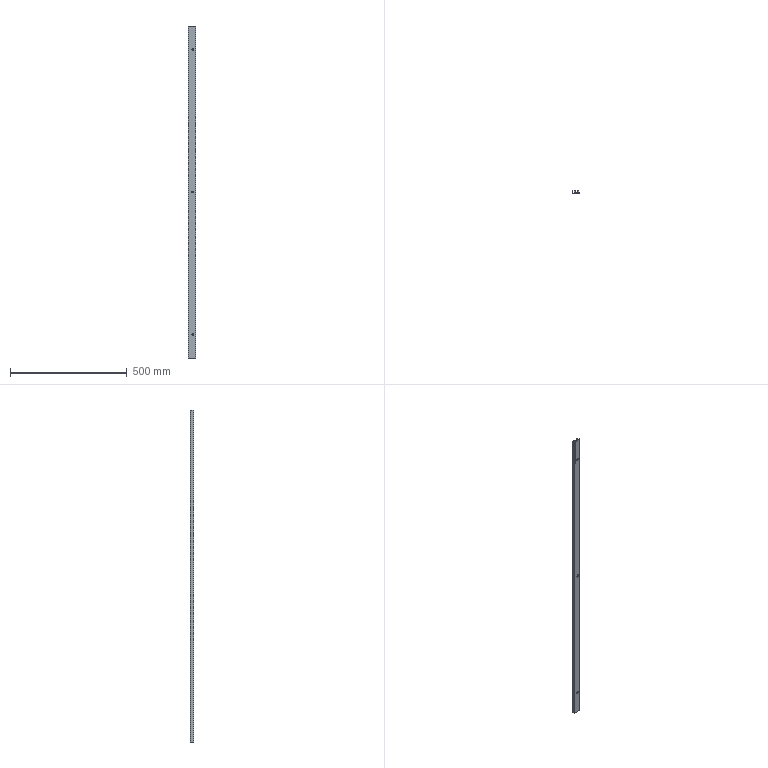Part | SolidWorks | features BaseBody 1, HoleWzd 1, ICE 1, MoveFace 1 | 1 solid | 31 faces | box 33.5 x 13.5 x 1420 mm | volume 265656 mm3 | plane 16 | cylinder 9 | cone 6 | commonest cylinder face diameters 2 x3 13.44 x3 4 x2 1.5 x1
STEP:
#1=CARTESIAN_POINT('',(20.,0.,1223.72));
#2=VERTEX_POINT('',#1);
#3=CARTESIAN_POINT('',(20.,0.,1216.28));
#4=VERTEX_POINT('',#3);
#5=CARTESIAN_POINT('',(20.,0.,1220.));
#6=DIRECTION('',(0.,-1.,0.));
#7=DIRECTION('',(0.,0.,-1.));
#8=AXIS2_PLACEMENT_3D('',#5,#6,#7);
#9=CIRCLE('',#8,3.72);
#10=EDGE_CURVE('',#2,#4,#9,.T.);
#11=ORIENTED_EDGE('',*,*,#10,.T.);
#12=CARTESIAN_POINT('',(20.,3.,1213.28));
#13=VERTEX_POINT('',#12);
#14=CARTESIAN_POINT('',(20.,3.,1213.28));
#15=DIRECTION('',(0.,0.7071,-0.7071));
#16=VECTOR('',#15,1000.);
#17=LINE('',#14,#16);
#18=EDGE_CURVE('',#4,#13,#17,.T.);
#19=ORIENTED_EDGE('',*,*,#18,.T.);
#20=CARTESIAN_POINT('',(20.,3.,1226.72));
#21=VERTEX_POINT('',#20);
#22=CARTESIAN_POINT('',(20.,3.,1220.));
#23=DIRECTION('',(0.,1.,0.));
#24=DIRECTION('',(0.,0.,1.));
#25=AXIS2_PLACEMENT_3D('',#22,#23,#24);
#26=CIRCLE('',#25,6.72);
#27=EDGE_CURVE('',#13,#21,#26,.T.);
#28=ORIENTED_EDGE('',*,*,#27,.T.);
#29=CARTESIAN_POINT('',(20.,3.,1226.72));
#30=DIRECTION('',(0.,0.7071,0.7071));
#31=VECTOR('',#30,1000.);
#32=LINE('',#29,#31);
#33=EDGE_CURVE('',#2,#21,#32,.T.);
#34=ORIENTED_EDGE('',*,*,#33,.F.);
#35=EDGE_LOOP('',(#11,#19,#28,#34));
#36=FACE_OUTER_BOUND('',#35,.T.);
#37=CARTESIAN_POINT('',(20.,3.,1220.));
#38=DIRECTION('',(0.,1.,0.));
#39=DIRECTION('',(0.,0.,1.));
#40=AXIS2_PLACEMENT_3D('',#37,#38,#39);
#41=CONICAL_SURFACE('',#40,6.72,0.7854);
#42=ADVANCED_FACE('',(#36),#41,.F.);
#43=CARTESIAN_POINT('',(20.,0.,3.72));
#44=VERTEX_POINT('',#43);
#45=CARTESIAN_POINT('',(20.,0.,-3.72));
#46=VERTEX_POINT('',#45);
#47=CARTESIAN_POINT('',(20.,0.,0.));
#48=DIRECTION('',(0.,-1.,0.));
#49=DIRECTION('',(0.,0.,-1.));
#50=AXIS2_PLACEMENT_3D('',#47,#48,#49);
#51=CIRCLE('',#50,3.72);
#52=EDGE_CURVE('',#44,#46,#51,.T.);
#53=ORIENTED_EDGE('',*,*,#52,.T.);
#54=CARTESIAN_POINT('',(20.,3.,-6.72));
#55=VERTEX_POINT('',#54);
#56=CARTESIAN_POINT('',(20.,3.,-6.72));
#57=DIRECTION('',(0.,0.7071,-0.7071));
#58=VECTOR('',#57,1000.);
#59=LINE('',#56,#58);
#60=EDGE_CURVE('',#46,#55,#59,.T.);
#61=ORIENTED_EDGE('',*,*,#60,.T.);
#62=CARTESIAN_POINT('',(20.,3.,6.72));
#63=VERTEX_POINT('',#62);
#64=CARTESIAN_POINT('',(20.,3.,0.));
#65=DIRECTION('',(0.,1.,0.));
#66=DIRECTION('',(0.,0.,1.));
#67=AXIS2_PLACEMENT_3D('',#64,#65,#66);
#68=CIRCLE('',#67,6.72);
#69=EDGE_CURVE('',#55,#63,#68,.T.);
#70=ORIENTED_EDGE('',*,*,#69,.T.);
#71=CARTESIAN_POINT('',(20.,3.,6.72));
#72=DIRECTION('',(0.,0.7071,0.7071));
#73=VECTOR('',#72,1000.);
#74=LINE('',#71,#73);
#75=EDGE_CURVE('',#44,#63,#74,.T.);
#76=ORIENTED_EDGE('',*,*,#75,.F.);
#77=EDGE_LOOP('',(#53,#61,#70,#76));
#78=FACE_OUTER_BOUND('',#77,.T.);
#79=CARTESIAN_POINT('',(20.,3.,0.));
#80=DIRECTION('',(0.,1.,0.));
#81=DIRECTION('',(0.,0.,1.));
#82=AXIS2_PLACEMENT_3D('',#79,#80,#81);
#83=CONICAL_SURFACE('',#82,6.72,0.7854);
#84=ADVANCED_FACE('',(#78),#83,.F.);
#85=CARTESIAN_POINT('',(20.,0.,613.72));
#86=VERTEX_POINT('',#85);
#87=CARTESIAN_POINT('',(20.,0.,606.28));
#88=VERTEX_POINT('',#87);
#89=CARTESIAN_POINT('',(20.,0.,610.));
#90=DIRECTION('',(0.,-1.,0.));
#91=DIRECTION('',(0.,0.,-1.));
#92=AXIS2_PLACEMENT_3D('',#89,#90,#91);
#93=CIRCLE('',#92,3.72);
#94=EDGE_CURVE('',#86,#88,#93,.T.);
#95=ORIENTED_EDGE('',*,*,#94,.T.);
#96=CARTESIAN_POINT('',(20.,3.,603.28));
#97=VERTEX_POINT('',#96);
#98=CARTESIAN_POINT('',(20.,3.,603.28));
#99=DIRECTION('',(0.,0.7071,-0.7071));
#100=VECTOR('',#99,1000.);
#101=LINE('',#98,#100);
#102=EDGE_CURVE('',#88,#97,#101,.T.);
#103=ORIENTED_EDGE('',*,*,#102,.T.);
#104=CARTESIAN_POINT('',(20.,3.,616.72));
#105=VERTEX_POINT('',#104);
#106=CARTESIAN_POINT('',(20.,3.,610.));
#107=DIRECTION('',(0.,1.,0.));
#108=DIRECTION('',(0.,0.,1.));
#109=AXIS2_PLACEMENT_3D('',#106,#107,#108);
#110=CIRCLE('',#109,6.72);
#111=EDGE_CURVE('',#97,#105,#110,.T.);
#112=ORIENTED_EDGE('',*,*,#111,.T.);
#113=CARTESIAN_POINT('',(20.,3.,616.72));
#114=DIRECTION('',(0.,0.7071,0.7071));
#115=VECTOR('',#114,1000.);
#116=LINE('',#113,#115);
#117=EDGE_CURVE('',#86,#105,#116,.T.);
#118=ORIENTED_EDGE('',*,*,#117,.F.);
#119=EDGE_LOOP('',(#95,#103,#112,#118));
#120=FACE_OUTER_BOUND('',#119,.T.);
#121=CARTESIAN_POINT('',(20.,3.,610.));
#122=DIRECTION('',(0.,1.,0.));
#123=DIRECTION('',(0.,0.,1.));
#124=AXIS2_PLACEMENT_3D('',#121,#122,#123);
#125=CONICAL_SURFACE('',#124,6.72,0.7854);
#126=ADVANCED_FACE('',(#120),#125,.F.);
#127=CARTESIAN_POINT('',(24.5,10.5,-4.991));
#128=VERTEX_POINT('',#127);
#129=CARTESIAN_POINT('',(24.5,10.5,-100.));
#130=VERTEX_POINT('',#129);
#131=CARTESIAN_POINT('',(24.5,10.5,-100.));
#132=DIRECTION('',(0.,0.,-1.));
#133=VECTOR('',#132,1000.);
#134=LINE('',#131,#133);
#135=EDGE_CURVE('',#128,#130,#134,.T.);
#136=ORIENTED_EDGE('',*,*,#135,.F.);
#137=CARTESIAN_POINT('',(24.5,10.5,4.991));
#138=VERTEX_POINT('',#137);
#139=CARTESIAN_POINT('',(24.5,10.5,-4.991));
#140=CARTESIAN_POINT('',(24.5,10.638,-4.991));
#141=CARTESIAN_POINT('',(24.515,10.777,-4.978));
#142=CARTESIAN_POINT('',(24.57,11.043,-4.927));
#143=CARTESIAN_POINT('',(24.611,11.171,-4.889));
#144=CARTESIAN_POINT('',(24.765,11.529,-4.74));
#145=CARTESIAN_POINT('',(24.907,11.728,-4.597));
#146=CARTESIAN_POINT('',(25.205,12.04,-4.256));
#147=CARTESIAN_POINT('',(25.365,12.156,-4.055));
#148=CARTESIAN_POINT('',(25.663,12.325,-3.627));
#149=CARTESIAN_POINT('',(25.806,12.38,-3.395));
#150=CARTESIAN_POINT('',(26.19,12.494,-2.672));
#151=CARTESIAN_POINT('',(26.387,12.501,-2.161));
#152=CARTESIAN_POINT('',(26.654,12.499,-1.091));
#153=CARTESIAN_POINT('',(26.72,12.488,-0.5481));
#154=CARTESIAN_POINT('',(26.72,12.488,0.2773));
#155=CARTESIAN_POINT('',(26.703,12.49,0.5529));
#156=CARTESIAN_POINT('',(26.636,12.496,1.095));
#157=CARTESIAN_POINT('',(26.586,12.499,1.362));
#158=CARTESIAN_POINT('',(26.388,12.501,2.155));
#159=CARTESIAN_POINT('',(26.188,12.493,2.677));
#160=CARTESIAN_POINT('',(25.805,12.38,3.396));
#161=CARTESIAN_POINT('',(25.662,12.324,3.629));
#162=CARTESIAN_POINT('',(25.438,12.197,3.95));
#163=CARTESIAN_POINT('',(25.362,12.147,4.053));
#164=CARTESIAN_POINT('',(25.208,12.03,4.249));
#165=CARTESIAN_POINT('',(25.13,11.961,4.342));
#166=CARTESIAN_POINT('',(24.98,11.805,4.513));
#167=CARTESIAN_POINT('',(24.908,11.717,4.591));
#168=CARTESIAN_POINT('',(24.774,11.518,4.73));
#169=CARTESIAN_POINT('',(24.714,11.408,4.79));
#170=CARTESIAN_POINT('',(24.612,11.172,4.888));
#171=CARTESIAN_POINT('',(24.57,11.043,4.927));
#172=CARTESIAN_POINT('',(24.515,10.778,4.978));
#173=CARTESIAN_POINT('',(24.5,10.64,4.991));
#174=CARTESIAN_POINT('',(24.5,10.5,4.991));
#175=B_SPLINE_CURVE_WITH_KNOTS('',3,(#139,#140,#141,#142,#143,#144,#145,#146,#147,#148,#149,#150,#151,#152,#153,#154,#155,#156,#157,#158,#159,#160,#161,#162,#163,#164,#165,#166,#167,#168,#169,#170,#171,#172,#173,#174),.UNSPECIFIED.,.F.,.F.,(4,2,2,2,2,2,2,2,2,2,2,2,2,2,2,2,2,4),(0.01321,0.01362,0.01403,0.01486,0.01569,0.01651,0.01816,0.01981,0.02064,0.02146,0.02311,0.02394,0.02435,0.02477,0.02518,0.02559,0.026,0.02642),.UNSPECIFIED.);
#176=EDGE_CURVE('',#128,#138,#175,.T.);
#177=ORIENTED_EDGE('',*,*,#176,.T.);
#178=CARTESIAN_POINT('',(24.5,10.5,605.009));
#179=VERTEX_POINT('',#178);
#180=CARTESIAN_POINT('',(24.5,10.5,-100.));
#181=DIRECTION('',(0.,0.,-1.));
#182=VECTOR('',#181,1000.);
#183=LINE('',#180,#182);
#184=EDGE_CURVE('',#179,#138,#183,.T.);
#185=ORIENTED_EDGE('',*,*,#184,.F.);
#186=CARTESIAN_POINT('',(24.5,10.5,614.991));
#187=VERTEX_POINT('',#186);
#188=CARTESIAN_POINT('',(24.5,10.5,605.009));
#189=CARTESIAN_POINT('',(24.5,10.638,605.009));
#190=CARTESIAN_POINT('',(24.515,10.777,605.022));
#191=CARTESIAN_POINT('',(24.57,11.043,605.073));
#192=CARTESIAN_POINT('',(24.611,11.171,605.111));
#193=CARTESIAN_POINT('',(24.765,11.529,605.26));
#194=CARTESIAN_POINT('',(24.907,11.728,605.403));
#195=CARTESIAN_POINT('',(25.205,12.04,605.744));
#196=CARTESIAN_POINT('',(25.365,12.156,605.945));
#197=CARTESIAN_POINT('',(25.663,12.325,606.373));
#198=CARTESIAN_POINT('',(25.806,12.38,606.605));
#199=CARTESIAN_POINT('',(26.19,12.494,607.328));
#200=CARTESIAN_POINT('',(26.387,12.501,607.839));
#201=CARTESIAN_POINT('',(26.654,12.499,608.909));
#202=CARTESIAN_POINT('',(26.72,12.488,609.452));
#203=CARTESIAN_POINT('',(26.72,12.488,610.277));
#204=CARTESIAN_POINT('',(26.703,12.49,610.553));
#205=CARTESIAN_POINT('',(26.636,12.496,611.095));
#206=CARTESIAN_POINT('',(26.586,12.499,611.362));
#207=CARTESIAN_POINT('',(26.388,12.501,612.155));
#208=CARTESIAN_POINT('',(26.188,12.493,612.677));
#209=CARTESIAN_POINT('',(25.805,12.38,613.396));
#210=CARTESIAN_POINT('',(25.662,12.324,613.629));
#211=CARTESIAN_POINT('',(25.438,12.197,613.95));
#212=CARTESIAN_POINT('',(25.362,12.147,614.053));
#213=CARTESIAN_POINT('',(25.208,12.03,614.249));
#214=CARTESIAN_POINT('',(25.13,11.961,614.342));
#215=CARTESIAN_POINT('',(24.98,11.805,614.513));
#216=CARTESIAN_POINT('',(24.908,11.717,614.591));
#217=CARTESIAN_POINT('',(24.774,11.518,614.73));
#218=CARTESIAN_POINT('',(24.714,11.408,614.79));
#219=CARTESIAN_POINT('',(24.612,11.172,614.888));
#220=CARTESIAN_POINT('',(24.57,11.043,614.927));
#221=CARTESIAN_POINT('',(24.515,10.778,614.978));
#222=CARTESIAN_POINT('',(24.5,10.64,614.991));
#223=CARTESIAN_POINT('',(24.5,10.5,614.991));
#224=B_SPLINE_CURVE_WITH_KNOTS('',3,(#188,#189,#190,#191,#192,#193,#194,#195,#196,#197,#198,#199,#200,#201,#202,#203,#204,#205,#206,#207,#208,#209,#210,#211,#212,#213,#214,#215,#216,#217,#218,#219,#220,#221,#222,#223),.UNSPECIFIED.,.F.,.F.,(4,2,2,2,2,2,2,2,2,2,2,2,2,2,2,2,2,4),(0.01321,0.01362,0.01403,0.01486,0.01569,0.01651,0.01816,0.01981,0.02064,0.02146,0.02311,0.02394,0.02435,0.02477,0.02518,0.02559,0.026,0.02642),.UNSPECIFIED.);
#225=EDGE_CURVE('',#179,#187,#224,.T.);
#226=ORIENTED_EDGE('',*,*,#225,.T.);
#227=CARTESIAN_POINT('',(24.5,10.5,1215.009));
#228=VERTEX_POINT('',#227);
#229=CARTESIAN_POINT('',(24.5,10.5,-100.));
#230=DIRECTION('',(0.,0.,-1.));
#231=VECTOR('',#230,1000.);
#232=LINE('',#229,#231);
#233=EDGE_CURVE('',#228,#187,#232,.T.);
#234=ORIENTED_EDGE('',*,*,#233,.F.);
#235=CARTESIAN_POINT('',(24.5,10.5,1224.991));
#236=VERTEX_POINT('',#235);
#237=CARTESIAN_POINT('',(24.5,10.5,1215.009));
#238=CARTESIAN_POINT('',(24.5,10.64,1215.009));
#239=CARTESIAN_POINT('',(24.514,10.776,1215.022));
#240=CARTESIAN_POINT('',(24.57,11.042,1215.073));
#241=CARTESIAN_POINT('',(24.611,11.171,1215.111));
#242=CARTESIAN_POINT('',(24.713,11.408,1215.209));
#243=CARTESIAN_POINT('',(24.775,11.519,1215.27));
#244=CARTESIAN_POINT('',(24.908,11.717,1215.409));
#245=CARTESIAN_POINT('',(24.981,11.806,1215.488));
#246=CARTESIAN_POINT('',(25.207,12.042,1215.746));
#247=CARTESIAN_POINT('',(25.363,12.155,1215.942));
#248=CARTESIAN_POINT('',(25.665,12.326,1216.376));
#249=CARTESIAN_POINT('',(25.806,12.38,1216.605));
#250=CARTESIAN_POINT('',(26.061,12.456,1217.084));
#251=CARTESIAN_POINT('',(26.176,12.476,1217.337));
#252=CARTESIAN_POINT('',(26.372,12.498,1217.849));
#253=CARTESIAN_POINT('',(26.454,12.501,1218.109));
#254=CARTESIAN_POINT('',(26.586,12.499,1218.638));
#255=CARTESIAN_POINT('',(26.636,12.496,1218.907));
#256=CARTESIAN_POINT('',(26.703,12.49,1219.453));
#257=CARTESIAN_POINT('',(26.72,12.488,1219.729));
#258=CARTESIAN_POINT('',(26.72,12.488,1220.275));
#259=CARTESIAN_POINT('',(26.703,12.49,1220.547));
#260=CARTESIAN_POINT('',(26.637,12.496,1221.089));
#261=CARTESIAN_POINT('',(26.587,12.499,1221.36));
#262=CARTESIAN_POINT('',(26.387,12.501,1222.161));
#263=CARTESIAN_POINT('',(26.191,12.494,1222.671));
#264=CARTESIAN_POINT('',(25.805,12.38,1223.396));
#265=CARTESIAN_POINT('',(25.663,12.325,1223.627));
#266=CARTESIAN_POINT('',(25.364,12.155,1224.057));
#267=CARTESIAN_POINT('',(25.205,12.039,1224.256));
#268=CARTESIAN_POINT('',(24.981,11.805,1224.512));
#269=CARTESIAN_POINT('',(24.907,11.716,1224.592));
#270=CARTESIAN_POINT('',(24.774,11.518,1224.73));
#271=CARTESIAN_POINT('',(24.714,11.409,1224.79));
#272=CARTESIAN_POINT('',(24.611,11.17,1224.889));
#273=CARTESIAN_POINT('',(24.571,11.044,1224.926));
#274=CARTESIAN_POINT('',(24.515,10.78,1224.977));
#275=CARTESIAN_POINT('',(24.5,10.64,1224.991));
#276=CARTESIAN_POINT('',(24.5,10.5,1224.991));
#277=B_SPLINE_CURVE_WITH_KNOTS('',3,(#237,#238,#239,#240,#241,#242,#243,#244,#245,#246,#247,#248,#249,#250,#251,#252,#253,#254,#255,#256,#257,#258,#259,#260,#261,#262,#263,#264,#265,#266,#267,#268,#269,#270,#271,#272,#273,#274,#275,#276),.UNSPECIFIED.,.F.,.F.,(4,2,2,2,2,2,2,2,2,2,2,2,2,2,2,2,2,2,2,4),(0.,0.0004127,0.0008255,0.001238,0.001651,0.002476,0.003302,0.004127,0.004953,0.005778,0.006604,0.007429,0.008255,0.009906,0.01073,0.01156,0.01197,0.01238,0.01279,0.01321),.UNSPECIFIED.);
#278=EDGE_CURVE('',#228,#236,#277,.T.);
#279=ORIENTED_EDGE('',*,*,#278,.T.);
#280=CARTESIAN_POINT('',(24.5,10.5,1320.));
#281=VERTEX_POINT('',#280);
#282=CARTESIAN_POINT('',(24.5,10.5,-100.));
#283=DIRECTION('',(0.,0.,-1.));
#284=VECTOR('',#283,1000.);
#285=LINE('',#282,#284);
#286=EDGE_CURVE('',#281,#236,#285,.T.);
#287=ORIENTED_EDGE('',*,*,#286,.F.);
#288=CARTESIAN_POINT('',(28.5,10.5,1320.));
#289=VERTEX_POINT('',#288);
#290=CARTESIAN_POINT('',(26.5,10.5,1320.));
#291=DIRECTION('',(0.,0.,1.));
#292=DIRECTION('',(1.,0.,0.));
#293=AXIS2_PLACEMENT_3D('',#290,#291,#292);
#294=CIRCLE('',#293,2.);
#295=EDGE_CURVE('',#289,#281,#294,.T.);
#296=ORIENTED_EDGE('',*,*,#295,.F.);
#297=CARTESIAN_POINT('',(28.5,10.5,-100.));
#298=VERTEX_POINT('',#297);
#299=CARTESIAN_POINT('',(28.5,10.5,-100.));
#300=DIRECTION('',(0.,0.,-1.));
#301=VECTOR('',#300,1000.);
#302=LINE('',#299,#301);
#303=EDGE_CURVE('',#289,#298,#302,.T.);
#304=ORIENTED_EDGE('',*,*,#303,.T.);
#305=CARTESIAN_POINT('',(26.5,10.5,-100.));
#306=DIRECTION('',(0.,0.,1.));
#307=DIRECTION('',(-1.,0.,0.));
#308=AXIS2_PLACEMENT_3D('',#305,#306,#307);
#309=CIRCLE('',#308,2.);
#310=EDGE_CURVE('',#298,#130,#309,.T.);
#311=ORIENTED_EDGE('',*,*,#310,.T.);
#312=EDGE_LOOP('',(#136,#177,#185,#226,#234,#279,#287,#296,#304,#311));
#313=FACE_OUTER_BOUND('',#312,.T.);
#314=CARTESIAN_POINT('',(26.5,10.5,-100.));
#315=DIRECTION('',(0.,0.,-1.));
#316=DIRECTION('',(-1.,0.,0.));
#317=AXIS2_PLACEMENT_3D('',#314,#315,#316);
#318=CYLINDRICAL_SURFACE('',#317,2.);
#319=ADVANCED_FACE('',(#313),#318,.T.);
#320=CARTESIAN_POINT('',(24.5,3.,-4.991));
#321=VERTEX_POINT('',#320);
#322=CARTESIAN_POINT('',(24.5,3.,-100.));
#323=VERTEX_POINT('',#322);
#324=CARTESIAN_POINT('',(24.5,3.,-100.));
#325=DIRECTION('',(0.,0.,-1.));
#326=VECTOR('',#325,1000.);
#327=LINE('',#324,#326);
#328=EDGE_CURVE('',#321,#323,#327,.T.);
#329=ORIENTED_EDGE('',*,*,#328,.F.);
#330=CARTESIAN_POINT('',(24.5,13.5,-4.991));
#331=DIRECTION('',(0.,1.,0.));
#332=VECTOR('',#331,1000.);
#333=LINE('',#330,#332);
#334=EDGE_CURVE('',#321,#128,#333,.T.);
#335=ORIENTED_EDGE('',*,*,#334,.T.);
#336=ORIENTED_EDGE('',*,*,#135,.T.);
#337=CARTESIAN_POINT('',(24.5,1.,-100.));
#338=DIRECTION('',(0.,-1.,0.));
#339=VECTOR('',#338,1000.);
#340=LINE('',#337,#339);
#341=EDGE_CURVE('',#130,#323,#340,.T.);
#342=ORIENTED_EDGE('',*,*,#341,.T.);
#343=EDGE_LOOP('',(#329,#335,#336,#342));
#344=FACE_OUTER_BOUND('',#343,.T.);
#345=CARTESIAN_POINT('',(24.5,10.5,-100.));
#346=DIRECTION('',(-1.,0.,0.));
#347=DIRECTION('',(0.,0.,1.));
#348=AXIS2_PLACEMENT_3D('',#345,#346,#347);
#349=PLANE('',#348);
#350=ADVANCED_FACE('',(#344),#349,.T.);
#351=ORIENTED_EDGE('',*,*,#184,.T.);
#352=CARTESIAN_POINT('',(24.5,3.,4.991));
#353=VERTEX_POINT('',#352);
#354=CARTESIAN_POINT('',(24.5,13.5,4.991));
#355=DIRECTION('',(0.,-1.,0.));
#356=VECTOR('',#355,1000.);
#357=LINE('',#354,#356);
#358=EDGE_CURVE('',#138,#353,#357,.T.);
#359=ORIENTED_EDGE('',*,*,#358,.T.);
#360=CARTESIAN_POINT('',(24.5,3.,605.009));
#361=VERTEX_POINT('',#360);
#362=CARTESIAN_POINT('',(24.5,3.,-100.));
#363=DIRECTION('',(0.,0.,-1.));
#364=VECTOR('',#363,1000.);
#365=LINE('',#362,#364);
#366=EDGE_CURVE('',#361,#353,#365,.T.);
#367=ORIENTED_EDGE('',*,*,#366,.F.);
#368=CARTESIAN_POINT('',(24.5,13.5,605.009));
#369=DIRECTION('',(0.,1.,0.));
#370=VECTOR('',#369,1000.);
#371=LINE('',#368,#370);
#372=EDGE_CURVE('',#361,#179,#371,.T.);
#373=ORIENTED_EDGE('',*,*,#372,.T.);
#374=EDGE_LOOP('',(#351,#359,#367,#373));
#375=FACE_OUTER_BOUND('',#374,.T.);
#376=CARTESIAN_POINT('',(24.5,10.5,-100.));
#377=DIRECTION('',(-1.,0.,0.));
#378=DIRECTION('',(0.,0.,1.));
#379=AXIS2_PLACEMENT_3D('',#376,#377,#378);
#380=PLANE('',#379);
#381=ADVANCED_FACE('',(#375),#380,.T.);
#382=ORIENTED_EDGE('',*,*,#233,.T.);
#383=CARTESIAN_POINT('',(24.5,3.,614.991));
#384=VERTEX_POINT('',#383);
#385=CARTESIAN_POINT('',(24.5,13.5,614.991));
#386=DIRECTION('',(0.,-1.,0.));
#387=VECTOR('',#386,1000.);
#388=LINE('',#385,#387);
#389=EDGE_CURVE('',#187,#384,#388,.T.);
#390=ORIENTED_EDGE('',*,*,#389,.T.);
#391=CARTESIAN_POINT('',(24.5,3.,1215.009));
#392=VERTEX_POINT('',#391);
#393=CARTESIAN_POINT('',(24.5,3.,-100.));
#394=DIRECTION('',(0.,0.,-1.));
#395=VECTOR('',#394,1000.);
#396=LINE('',#393,#395);
#397=EDGE_CURVE('',#392,#384,#396,.T.);
#398=ORIENTED_EDGE('',*,*,#397,.F.);
#399=CARTESIAN_POINT('',(24.5,13.5,1215.009));
#400=DIRECTION('',(0.,1.,0.));
#401=VECTOR('',#400,1000.);
#402=LINE('',#399,#401);
#403=EDGE_CURVE('',#392,#228,#402,.T.);
#404=ORIENTED_EDGE('',*,*,#403,.T.);
#405=EDGE_LOOP('',(#382,#390,#398,#404));
#406=FACE_OUTER_BOUND('',#405,.T.);
#407=CARTESIAN_POINT('',(24.5,10.5,-100.));
#408=DIRECTION('',(-1.,0.,0.));
#409=DIRECTION('',(0.,0.,1.));
#410=AXIS2_PLACEMENT_3D('',#407,#408,#409);
#411=PLANE('',#410);
#412=ADVANCED_FACE('',(#406),#411,.T.);
#413=ORIENTED_EDGE('',*,*,#286,.T.);
#414=CARTESIAN_POINT('',(24.5,3.,1224.991));
#415=VERTEX_POINT('',#414);
#416=CARTESIAN_POINT('',(24.5,13.5,1224.991));
#417=DIRECTION('',(0.,-1.,0.));
#418=VECTOR('',#417,1000.);
#419=LINE('',#416,#418);
#420=EDGE_CURVE('',#236,#415,#419,.T.);
#421=ORIENTED_EDGE('',*,*,#420,.T.);
#422=CARTESIAN_POINT('',(24.5,3.,1320.));
#423=VERTEX_POINT('',#422);
#424=CARTESIAN_POINT('',(24.5,3.,-100.));
#425=DIRECTION('',(0.,0.,-1.));
#426=VECTOR('',#425,1000.);
#427=LINE('',#424,#426);
#428=EDGE_CURVE('',#423,#415,#427,.T.);
#429=ORIENTED_EDGE('',*,*,#428,.F.);
#430=CARTESIAN_POINT('',(24.5,1.,1320.));
#431=DIRECTION('',(0.,-1.,0.));
#432=VECTOR('',#431,1000.);
#433=LINE('',#430,#432);
#434=EDGE_CURVE('',#281,#423,#433,.T.);
#435=ORIENTED_EDGE('',*,*,#434,.F.);
#436=EDGE_LOOP('',(#413,#421,#429,#435));
#437=FACE_OUTER_BOUND('',#436,.T.);
#438=CARTESIAN_POINT('',(24.5,10.5,-100.));
#439=DIRECTION('',(-1.,0.,0.));
#440=DIRECTION('',(0.,0.,1.));
#441=AXIS2_PLACEMENT_3D('',#438,#439,#440);
#442=PLANE('',#441);
#443=ADVANCED_FACE('',(#437),#442,.T.);
#444=ORIENTED_EDGE('',*,*,#10,.F.);
#445=CARTESIAN_POINT('',(20.,0.,1220.));
#446=DIRECTION('',(0.,-1.,0.));
#447=DIRECTION('',(0.,0.,-1.));
#448=AXIS2_PLACEMENT_3D('',#445,#446,#447);
#449=CIRCLE('',#448,3.72);
#450=EDGE_CURVE('',#4,#2,#449,.T.);
#451=ORIENTED_EDGE('',*,*,#450,.F.);
#452=EDGE_LOOP('',(#444,#451));
#453=FACE_BOUND('',#452,.T.);
#454=ORIENTED_EDGE('',*,*,#94,.F.);
#455=CARTESIAN_POINT('',(20.,0.,610.));
#456=DIRECTION('',(0.,-1.,0.));
#457=DIRECTION('',(0.,0.,-1.));
#458=AXIS2_PLACEMENT_3D('',#455,#456,#457);
#459=CIRCLE('',#458,3.72);
#460=EDGE_CURVE('',#88,#86,#459,.T.);
#461=ORIENTED_EDGE('',*,*,#460,.F.);
#462=EDGE_LOOP('',(#454,#461));
#463=FACE_BOUND('',#462,.T.);
#464=CARTESIAN_POINT('',(1.,0.,-100.));
#465=VERTEX_POINT('',#464);
#466=CARTESIAN_POINT('',(32.5,0.,-100.));
#467=VERTEX_POINT('',#466);
#468=CARTESIAN_POINT('',(1.,0.,-100.));
#469=DIRECTION('',(1.,0.,0.));
#470=VECTOR('',#469,1000.);
#471=LINE('',#468,#470);
#472=EDGE_CURVE('',#465,#467,#471,.T.);
#473=ORIENTED_EDGE('',*,*,#472,.T.);
#474=CARTESIAN_POINT('',(32.5,0.,1320.));
#475=VERTEX_POINT('',#474);
#476=CARTESIAN_POINT('',(32.5,0.,-100.));
#477=DIRECTION('',(0.,0.,1.));
#478=VECTOR('',#477,1000.);
#479=LINE('',#476,#478);
#480=EDGE_CURVE('',#467,#475,#479,.T.);
#481=ORIENTED_EDGE('',*,*,#480,.T.);
#482=CARTESIAN_POINT('',(1.,0.,1320.));
#483=VERTEX_POINT('',#482);
#484=CARTESIAN_POINT('',(1.,0.,1320.));
#485=DIRECTION('',(-1.,0.,0.));
#486=VECTOR('',#485,1000.);
#487=LINE('',#484,#486);
#488=EDGE_CURVE('',#475,#483,#487,.T.);
#489=ORIENTED_EDGE('',*,*,#488,.T.);
#490=CARTESIAN_POINT('',(1.,0.,-100.));
#491=DIRECTION('',(0.,0.,-1.));
#492=VECTOR('',#491,1000.);
#493=LINE('',#490,#492);
#494=EDGE_CURVE('',#483,#465,#493,.T.);
#495=ORIENTED_EDGE('',*,*,#494,.T.);
#496=EDGE_LOOP('',(#473,#481,#489,#495));
#497=FACE_OUTER_BOUND('',#496,.T.);
#498=ORIENTED_EDGE('',*,*,#52,.F.);
#499=CARTESIAN_POINT('',(20.,0.,0.));
#500=DIRECTION('',(0.,-1.,0.));
#501=DIRECTION('',(0.,0.,-1.));
#502=AXIS2_PLACEMENT_3D('',#499,#500,#501);
#503=CIRCLE('',#502,3.72);
#504=EDGE_CURVE('',#46,#44,#503,.T.);
#505=ORIENTED_EDGE('',*,*,#504,.F.);
#506=EDGE_LOOP('',(#498,#505));
#507=FACE_BOUND('',#506,.T.);
#508=CARTESIAN_POINT('',(1.,0.,-100.));
#509=DIRECTION('',(0.,-1.,0.));
#510=DIRECTION('',(0.,0.,-1.));
#511=AXIS2_PLACEMENT_3D('',#508,#509,#510);
#512=PLANE('',#511);
#513=ADVANCED_FACE('',(#453,#463,#497,#507),#512,.T.);
#514=CARTESIAN_POINT('',(33.5,1.,-100.));
#515=VERTEX_POINT('',#514);
#516=CARTESIAN_POINT('',(32.5,1.,-100.));
#517=DIRECTION('',(0.,0.,1.));
#518=DIRECTION('',(-1.,0.,0.));
#519=AXIS2_PLACEMENT_3D('',#516,#517,#518);
#520=CIRCLE('',#519,1.);
#521=EDGE_CURVE('',#467,#515,#520,.T.);
#522=ORIENTED_EDGE('',*,*,#521,.T.);
#523=CARTESIAN_POINT('',(33.5,1.,1320.));
#524=VERTEX_POINT('',#523);
#525=CARTESIAN_POINT('',(33.5,1.,-100.));
#526=DIRECTION('',(0.,0.,1.));
#527=VECTOR('',#526,1000.);
#528=LINE('',#525,#527);
#529=EDGE_CURVE('',#515,#524,#528,.T.);
#530=ORIENTED_EDGE('',*,*,#529,.T.);
#531=CARTESIAN_POINT('',(32.5,1.,1320.));
#532=DIRECTION('',(0.,0.,-1.));
#533=DIRECTION('',(1.,0.,0.));
#534=AXIS2_PLACEMENT_3D('',#531,#532,#533);
#535=CIRCLE('',#534,1.);
#536=EDGE_CURVE('',#524,#475,#535,.T.);
#537=ORIENTED_EDGE('',*,*,#536,.T.);
#538=ORIENTED_EDGE('',*,*,#480,.F.);
#539=EDGE_LOOP('',(#522,#530,#537,#538));
#540=FACE_OUTER_BOUND('',#539,.T.);
#541=CARTESIAN_POINT('',(32.5,1.,-100.));
#542=DIRECTION('',(0.,0.,-1.));
#543=DIRECTION('',(-1.,0.,0.));
#544=AXIS2_PLACEMENT_3D('',#541,#542,#543);
#545=CYLINDRICAL_SURFACE('',#544,1.);
#546=ADVANCED_FACE('',(#540),#545,.T.);
#547=CARTESIAN_POINT('',(1.5,12.75,-100.));
#548=VERTEX_POINT('',#547);
#549=CARTESIAN_POINT('',(0.,12.75,-100.));
#550=VERTEX_POINT('',#549);
#551=CARTESIAN_POINT('',(0.75,12.75,-100.));
#552=DIRECTION('',(0.,0.,1.));
#553=DIRECTION('',(-1.,0.,0.));
#554=AXIS2_PLACEMENT_3D('',#551,#552,#553);
#555=CIRCLE('',#554,0.75);
#556=EDGE_CURVE('',#548,#550,#555,.T.);
#557=ORIENTED_EDGE('',*,*,#556,.F.);
#558=CARTESIAN_POINT('',(1.5,3.,-100.));
#559=VERTEX_POINT('',#558);
#560=CARTESIAN_POINT('',(1.5,1.,-100.));
#561=DIRECTION('',(0.,1.,0.));
#562=VECTOR('',#561,1000.);
#563=LINE('',#560,#562);
#564=EDGE_CURVE('',#559,#548,#563,.T.);
#565=ORIENTED_EDGE('',*,*,#564,.F.);
#566=CARTESIAN_POINT('',(8.5,3.,-100.));
#567=VERTEX_POINT('',#566);
#568=CARTESIAN_POINT('',(1.,3.,-100.));
#569=DIRECTION('',(-1.,0.,0.));
#570=VECTOR('',#569,1000.);
#571=LINE('',#568,#570);
#572=EDGE_CURVE('',#567,#559,#571,.T.);
#573=ORIENTED_EDGE('',*,*,#572,.F.);
#574=CARTESIAN_POINT('',(8.5,10.5,-100.));
#575=VERTEX_POINT('',#574);
#576=CARTESIAN_POINT('',(8.5,1.,-100.));
#577=DIRECTION('',(0.,-1.,0.));
#578=VECTOR('',#577,1000.);
#579=LINE('',#576,#578);
#580=EDGE_CURVE('',#575,#567,#579,.T.);
#581=ORIENTED_EDGE('',*,*,#580,.F.);
#582=CARTESIAN_POINT('',(12.5,10.5,-100.));
#583=VERTEX_POINT('',#582);
#584=CARTESIAN_POINT('',(10.5,10.5,-100.));
#585=DIRECTION('',(0.,0.,1.));
#586=DIRECTION('',(-1.,0.,0.));
#587=AXIS2_PLACEMENT_3D('',#584,#585,#586);
#588=CIRCLE('',#587,2.);
#589=EDGE_CURVE('',#583,#575,#588,.T.);
#590=ORIENTED_EDGE('',*,*,#589,.F.);
#591=CARTESIAN_POINT('',(12.5,3.,-100.));
#592=VERTEX_POINT('',#591);
#593=CARTESIAN_POINT('',(12.5,1.,-100.));
#594=DIRECTION('',(0.,1.,0.));
#595=VECTOR('',#594,1000.);
#596=LINE('',#593,#595);
#597=EDGE_CURVE('',#592,#583,#596,.T.);
#598=ORIENTED_EDGE('',*,*,#597,.F.);
#599=CARTESIAN_POINT('',(1.,3.,-100.));
#600=DIRECTION('',(-1.,0.,0.));
#601=VECTOR('',#600,1000.);
#602=LINE('',#599,#601);
#603=EDGE_CURVE('',#323,#592,#602,.T.);
#604=ORIENTED_EDGE('',*,*,#603,.F.);
#605=ORIENTED_EDGE('',*,*,#341,.F.);
#606=ORIENTED_EDGE('',*,*,#310,.F.);
#607=CARTESIAN_POINT('',(28.5,3.,-100.));
#608=VERTEX_POINT('',#607);
#609=CARTESIAN_POINT('',(28.5,1.,-100.));
#610=DIRECTION('',(0.,1.,0.));
#611=VECTOR('',#610,1000.);
#612=LINE('',#609,#611);
#613=EDGE_CURVE('',#608,#298,#612,.T.);
#614=ORIENTED_EDGE('',*,*,#613,.F.);
#615=CARTESIAN_POINT('',(32.5,3.,-100.));
#616=VERTEX_POINT('',#615);
#617=CARTESIAN_POINT('',(1.,3.,-100.));
#618=DIRECTION('',(-1.,0.,0.));
#619=VECTOR('',#618,1000.);
#620=LINE('',#617,#619);
#621=EDGE_CURVE('',#616,#608,#620,.T.);
#622=ORIENTED_EDGE('',*,*,#621,.F.);
#623=CARTESIAN_POINT('',(33.5,2.,-100.));
#624=VERTEX_POINT('',#623);
#625=CARTESIAN_POINT('',(32.5,2.,-100.));
#626=DIRECTION('',(0.,0.,1.));
#627=DIRECTION('',(-1.,0.,0.));
#628=AXIS2_PLACEMENT_3D('',#625,#626,#627);
#629=CIRCLE('',#628,1.);
#630=EDGE_CURVE('',#624,#616,#629,.T.);
#631=ORIENTED_EDGE('',*,*,#630,.F.);
#632=CARTESIAN_POINT('',(33.5,1.,-100.));
#633=DIRECTION('',(0.,1.,0.));
#634=VECTOR('',#633,1000.);
#635=LINE('',#632,#634);
#636=EDGE_CURVE('',#515,#624,#635,.T.);
#637=ORIENTED_EDGE('',*,*,#636,.F.);
#638=ORIENTED_EDGE('',*,*,#521,.F.);
#639=ORIENTED_EDGE('',*,*,#472,.F.);
#640=CARTESIAN_POINT('',(0.,1.,-100.));
#641=VERTEX_POINT('',#640);
#642=CARTESIAN_POINT('',(1.,1.,-100.));
#643=DIRECTION('',(0.,0.,1.));
#644=DIRECTION('',(-1.,0.,0.));
#645=AXIS2_PLACEMENT_3D('',#642,#643,#644);
#646=CIRCLE('',#645,1.);
#647=EDGE_CURVE('',#641,#465,#646,.T.);
#648=ORIENTED_EDGE('',*,*,#647,.F.);
#649=CARTESIAN_POINT('',(0.,1.,-100.));
#650=DIRECTION('',(0.,-1.,0.));
#651=VECTOR('',#650,1000.);
#652=LINE('',#649,#651);
#653=EDGE_CURVE('',#550,#641,#652,.T.);
#654=ORIENTED_EDGE('',*,*,#653,.F.);
#655=EDGE_LOOP('',(#557,#565,#573,#581,#590,#598,#604,#605,#606,#614,#622,#631,#637,#638,#639,#648,#654));
#656=FACE_OUTER_BOUND('',#655,.T.);
#657=CARTESIAN_POINT('',(1.,1.,-100.));
#658=DIRECTION('',(0.,0.,1.));
#659=DIRECTION('',(1.,0.,0.));
#660=AXIS2_PLACEMENT_3D('',#657,#658,#659);
#661=PLANE('',#660);
#662=ADVANCED_FACE('',(#656),#661,.F.);
#663=ORIENTED_EDGE('',*,*,#647,.T.);
#664=ORIENTED_EDGE('',*,*,#494,.F.);
#665=CARTESIAN_POINT('',(0.,1.,1320.));
#666=VERTEX_POINT('',#665);
#667=CARTESIAN_POINT('',(1.,1.,1320.));
#668=DIRECTION('',(0.,0.,-1.));
#669=DIRECTION('',(1.,0.,0.));
#670=AXIS2_PLACEMENT_3D('',#667,#668,#669);
#671=CIRCLE('',#670,1.);
#672=EDGE_CURVE('',#483,#666,#671,.T.);
#673=ORIENTED_EDGE('',*,*,#672,.T.);
#674=CARTESIAN_POINT('',(0.,1.,-100.));
#675=DIRECTION('',(0.,0.,-1.));
#676=VECTOR('',#675,1000.);
#677=LINE('',#674,#676);
#678=EDGE_CURVE('',#666,#641,#677,.T.);
#679=ORIENTED_EDGE('',*,*,#678,.T.);
#680=EDGE_LOOP('',(#663,#664,#673,#679));
#681=FACE_OUTER_BOUND('',#680,.T.);
#682=CARTESIAN_POINT('',(1.,1.,-100.));
#683=DIRECTION('',(0.,0.,-1.));
#684=DIRECTION('',(-1.,0.,0.));
#685=AXIS2_PLACEMENT_3D('',#682,#683,#684);
#686=CYLINDRICAL_SURFACE('',#685,1.);
#687=ADVANCED_FACE('',(#681),#686,.T.);
#688=CARTESIAN_POINT('',(1.5,3.,1320.));
#689=VERTEX_POINT('',#688);
#690=CARTESIAN_POINT('',(1.5,12.75,1320.));
#691=VERTEX_POINT('',#690);
#692=CARTESIAN_POINT('',(1.5,1.,1320.));
#693=DIRECTION('',(0.,1.,0.));
#694=VECTOR('',#693,1000.);
#695=LINE('',#692,#694);
#696=EDGE_CURVE('',#689,#691,#695,.T.);
#697=ORIENTED_EDGE('',*,*,#696,.T.);
#698=CARTESIAN_POINT('',(0.,12.75,1320.));
#699=VERTEX_POINT('',#698);
#700=CARTESIAN_POINT('',(0.75,12.75,1320.));
#701=DIRECTION('',(0.,0.,1.));
#702=DIRECTION('',(1.,0.,0.));
#703=AXIS2_PLACEMENT_3D('',#700,#701,#702);
#704=CIRCLE('',#703,0.75);
#705=EDGE_CURVE('',#691,#699,#704,.T.);
#706=ORIENTED_EDGE('',*,*,#705,.T.);
#707=CARTESIAN_POINT('',(0.,1.,1320.));
#708=DIRECTION('',(0.,-1.,0.));
#709=VECTOR('',#708,1000.);
#710=LINE('',#707,#709);
#711=EDGE_CURVE('',#699,#666,#710,.T.);
#712=ORIENTED_EDGE('',*,*,#711,.T.);
#713=ORIENTED_EDGE('',*,*,#672,.F.);
#714=ORIENTED_EDGE('',*,*,#488,.F.);
#715=ORIENTED_EDGE('',*,*,#536,.F.);
#716=CARTESIAN_POINT('',(33.5,2.,1320.));
#717=VERTEX_POINT('',#716);
#718=CARTESIAN_POINT('',(33.5,1.,1320.));
#719=DIRECTION('',(0.,1.,0.));
#720=VECTOR('',#719,1000.);
#721=LINE('',#718,#720);
#722=EDGE_CURVE('',#524,#717,#721,.T.);
#723=ORIENTED_EDGE('',*,*,#722,.T.);
#724=CARTESIAN_POINT('',(32.5,3.,1320.));
#725=VERTEX_POINT('',#724);
#726=CARTESIAN_POINT('',(32.5,2.,1320.));
#727=DIRECTION('',(0.,0.,-1.));
#728=DIRECTION('',(1.,0.,0.));
#729=AXIS2_PLACEMENT_3D('',#726,#727,#728);
#730=CIRCLE('',#729,1.);
#731=EDGE_CURVE('',#725,#717,#730,.T.);
#732=ORIENTED_EDGE('',*,*,#731,.F.);
#733=CARTESIAN_POINT('',(28.5,3.,1320.));
#734=VERTEX_POINT('',#733);
#735=CARTESIAN_POINT('',(1.,3.,1320.));
#736=DIRECTION('',(-1.,0.,0.));
#737=VECTOR('',#736,1000.);
#738=LINE('',#735,#737);
#739=EDGE_CURVE('',#725,#734,#738,.T.);
#740=ORIENTED_EDGE('',*,*,#739,.T.);
#741=CARTESIAN_POINT('',(28.5,1.,1320.));
#742=DIRECTION('',(0.,1.,0.));
#743=VECTOR('',#742,1000.);
#744=LINE('',#741,#743);
#745=EDGE_CURVE('',#734,#289,#744,.T.);
#746=ORIENTED_EDGE('',*,*,#745,.T.);
#747=ORIENTED_EDGE('',*,*,#295,.T.);
#748=ORIENTED_EDGE('',*,*,#434,.T.);
#749=CARTESIAN_POINT('',(12.5,3.,1320.));
#750=VERTEX_POINT('',#749);
#751=CARTESIAN_POINT('',(1.,3.,1320.));
#752=DIRECTION('',(-1.,0.,0.));
#753=VECTOR('',#752,1000.);
#754=LINE('',#751,#753);
#755=EDGE_CURVE('',#423,#750,#754,.T.);
#756=ORIENTED_EDGE('',*,*,#755,.T.);
#757=CARTESIAN_POINT('',(12.5,10.5,1320.));
#758=VERTEX_POINT('',#757);
#759=CARTESIAN_POINT('',(12.5,1.,1320.));
#760=DIRECTION('',(0.,1.,0.));
#761=VECTOR('',#760,1000.);
#762=LINE('',#759,#761);
#763=EDGE_CURVE('',#750,#758,#762,.T.);
#764=ORIENTED_EDGE('',*,*,#763,.T.);
#765=CARTESIAN_POINT('',(8.5,10.5,1320.));
#766=VERTEX_POINT('',#765);
#767=CARTESIAN_POINT('',(10.5,10.5,1320.));
#768=DIRECTION('',(0.,0.,1.));
#769=DIRECTION('',(1.,0.,0.));
#770=AXIS2_PLACEMENT_3D('',#767,#768,#769);
#771=CIRCLE('',#770,2.);
#772=EDGE_CURVE('',#758,#766,#771,.T.);
#773=ORIENTED_EDGE('',*,*,#772,.T.);
#774=CARTESIAN_POINT('',(8.5,3.,1320.));
#775=VERTEX_POINT('',#774);
#776=CARTESIAN_POINT('',(8.5,1.,1320.));
#777=DIRECTION('',(0.,-1.,0.));
#778=VECTOR('',#777,1000.);
#779=LINE('',#776,#778);
#780=EDGE_CURVE('',#766,#775,#779,.T.);
#781=ORIENTED_EDGE('',*,*,#780,.T.);
#782=CARTESIAN_POINT('',(1.,3.,1320.));
#783=DIRECTION('',(-1.,0.,0.));
#784=VECTOR('',#783,1000.);
#785=LINE('',#782,#784);
#786=EDGE_CURVE('',#775,#689,#785,.T.);
#787=ORIENTED_EDGE('',*,*,#786,.T.);
#788=EDGE_LOOP('',(#697,#706,#712,#713,#714,#715,#723,#732,#740,#746,#747,#748,#756,#764,#773,#781,#787));
#789=FACE_OUTER_BOUND('',#788,.T.);
#790=CARTESIAN_POINT('',(1.,1.,1320.));
#791=DIRECTION('',(0.,0.,1.));
#792=DIRECTION('',(1.,0.,0.));
#793=AXIS2_PLACEMENT_3D('',#790,#791,#792);
#794=PLANE('',#793);
#795=ADVANCED_FACE('',(#789),#794,.T.);
#796=ORIENTED_EDGE('',*,*,#636,.T.);
#797=CARTESIAN_POINT('',(33.5,2.,-100.));
#798=DIRECTION('',(0.,0.,1.));
#799=VECTOR('',#798,1000.);
#800=LINE('',#797,#799);
#801=EDGE_CURVE('',#624,#717,#800,.T.);
#802=ORIENTED_EDGE('',*,*,#801,.T.);
#803=ORIENTED_EDGE('',*,*,#722,.F.);
#804=ORIENTED_EDGE('',*,*,#529,.F.);
#805=EDGE_LOOP('',(#796,#802,#803,#804));
#806=FACE_OUTER_BOUND('',#805,.T.);
#807=CARTESIAN_POINT('',(33.5,1.,-100.));
#808=DIRECTION('',(1.,0.,0.));
#809=DIRECTION('',(0.,0.,-1.));
#810=AXIS2_PLACEMENT_3D('',#807,#808,#809);
#811=PLANE('',#810);
#812=ADVANCED_FACE('',(#806),#811,.T.);
#813=ORIENTED_EDGE('',*,*,#653,.T.);
#814=ORIENTED_EDGE('',*,*,#678,.F.);
#815=ORIENTED_EDGE('',*,*,#711,.F.);
#816=CARTESIAN_POINT('',(0.,12.75,-100.));
#817=DIRECTION('',(0.,0.,-1.));
#818=VECTOR('',#817,1000.);
#819=LINE('',#816,#818);
#820=EDGE_CURVE('',#699,#550,#819,.T.);
#821=ORIENTED_EDGE('',*,*,#820,.T.);
#822=EDGE_LOOP('',(#813,#814,#815,#821));
#823=FACE_OUTER_BOUND('',#822,.T.);
#824=CARTESIAN_POINT('',(0.,12.75,-100.));
#825=DIRECTION('',(-1.,0.,0.));
#826=DIRECTION('',(0.,0.,1.));
#827=AXIS2_PLACEMENT_3D('',#824,#825,#826);
#828=PLANE('',#827);
#829=ADVANCED_FACE('',(#823),#828,.T.);
#830=ORIENTED_EDGE('',*,*,#556,.T.);
#831=ORIENTED_EDGE('',*,*,#820,.F.);
#832=ORIENTED_EDGE('',*,*,#705,.F.);
#833=CARTESIAN_POINT('',(1.5,12.75,-100.));
#834=DIRECTION('',(0.,0.,-1.));
#835=VECTOR('',#834,1000.);
#836=LINE('',#833,#835);
#837=EDGE_CURVE('',#691,#548,#836,.T.);
#838=ORIENTED_EDGE('',*,*,#837,.T.);
#839=EDGE_LOOP('',(#830,#831,#832,#838));
#840=FACE_OUTER_BOUND('',#839,.T.);
#841=CARTESIAN_POINT('',(0.75,12.75,-100.));
#842=DIRECTION('',(0.,0.,-1.));
#843=DIRECTION('',(-1.,0.,0.));
#844=AXIS2_PLACEMENT_3D('',#841,#842,#843);
#845=CYLINDRICAL_SURFACE('',#844,0.75);
#846=ADVANCED_FACE('',(#840),#845,.T.);
#847=ORIENTED_EDGE('',*,*,#564,.T.);
#848=ORIENTED_EDGE('',*,*,#837,.F.);
#849=ORIENTED_EDGE('',*,*,#696,.F.);
#850=CARTESIAN_POINT('',(1.5,3.,-100.));
#851=DIRECTION('',(0.,0.,-1.));
#852=VECTOR('',#851,1000.);
#853=LINE('',#850,#852);
#854=EDGE_CURVE('',#689,#559,#853,.T.);
#855=ORIENTED_EDGE('',*,*,#854,.T.);
#856=EDGE_LOOP('',(#847,#848,#849,#855));
#857=FACE_OUTER_BOUND('',#856,.T.);
#858=CARTESIAN_POINT('',(1.5,3.,-100.));
#859=DIRECTION('',(1.,0.,0.));
#860=DIRECTION('',(0.,0.,-1.));
#861=AXIS2_PLACEMENT_3D('',#858,#859,#860);
#862=PLANE('',#861);
#863=ADVANCED_FACE('',(#857),#862,.T.);
#864=ORIENTED_EDGE('',*,*,#572,.T.);
#865=ORIENTED_EDGE('',*,*,#854,.F.);
#866=ORIENTED_EDGE('',*,*,#786,.F.);
#867=CARTESIAN_POINT('',(8.5,3.,-100.));
#868=DIRECTION('',(0.,0.,-1.));
#869=VECTOR('',#868,1000.);
#870=LINE('',#867,#869);
#871=EDGE_CURVE('',#775,#567,#870,.T.);
#872=ORIENTED_EDGE('',*,*,#871,.T.);
#873=EDGE_LOOP('',(#864,#865,#866,#872));
#874=FACE_OUTER_BOUND('',#873,.T.);
#875=CARTESIAN_POINT('',(8.5,3.,-100.));
#876=DIRECTION('',(0.,1.,0.));
#877=DIRECTION('',(0.,0.,1.));
#878=AXIS2_PLACEMENT_3D('',#875,#876,#877);
#879=PLANE('',#878);
#880=ADVANCED_FACE('',(#874),#879,.T.);
#881=ORIENTED_EDGE('',*,*,#580,.T.);
#882=ORIENTED_EDGE('',*,*,#871,.F.);
#883=ORIENTED_EDGE('',*,*,#780,.F.);
#884=CARTESIAN_POINT('',(8.5,10.5,-100.));
#885=DIRECTION('',(0.,0.,-1.));
#886=VECTOR('',#885,1000.);
#887=LINE('',#884,#886);
#888=EDGE_CURVE('',#766,#575,#887,.T.);
#889=ORIENTED_EDGE('',*,*,#888,.T.);
#890=EDGE_LOOP('',(#881,#882,#883,#889));
#891=FACE_OUTER_BOUND('',#890,.T.);
#892=CARTESIAN_POINT('',(8.5,10.5,-100.));
#893=DIRECTION('',(-1.,0.,0.));
#894=DIRECTION('',(0.,0.,1.));
#895=AXIS2_PLACEMENT_3D('',#892,#893,#894);
#896=PLANE('',#895);
#897=ADVANCED_FACE('',(#891),#896,.T.);
#898=ORIENTED_EDGE('',*,*,#589,.T.);
#899=ORIENTED_EDGE('',*,*,#888,.F.);
#900=ORIENTED_EDGE('',*,*,#772,.F.);
#901=CARTESIAN_POINT('',(12.5,10.5,-100.));
#902=DIRECTION('',(0.,0.,-1.));
#903=VECTOR('',#902,1000.);
#904=LINE('',#901,#903);
#905=EDGE_CURVE('',#758,#583,#904,.T.);
#906=ORIENTED_EDGE('',*,*,#905,.T.);
#907=EDGE_LOOP('',(#898,#899,#900,#906));
#908=FACE_OUTER_BOUND('',#907,.T.);
#909=CARTESIAN_POINT('',(10.5,10.5,-100.));
#910=DIRECTION('',(0.,0.,-1.));
#911=DIRECTION('',(-1.,0.,0.));
#912=AXIS2_PLACEMENT_3D('',#909,#910,#911);
#913=CYLINDRICAL_SURFACE('',#912,2.);
#914=ADVANCED_FACE('',(#908),#913,.T.);
#915=ORIENTED_EDGE('',*,*,#597,.T.);
#916=ORIENTED_EDGE('',*,*,#905,.F.);
#917=ORIENTED_EDGE('',*,*,#763,.F.);
#918=CARTESIAN_POINT('',(12.5,3.,-100.));
#919=DIRECTION('',(0.,0.,-1.));
#920=VECTOR('',#919,1000.);
#921=LINE('',#918,#920);
#922=EDGE_CURVE('',#750,#592,#921,.T.);
#923=ORIENTED_EDGE('',*,*,#922,.T.);
#924=EDGE_LOOP('',(#915,#916,#917,#923));
#925=FACE_OUTER_BOUND('',#924,.T.);
#926=CARTESIAN_POINT('',(12.5,3.,-100.));
#927=DIRECTION('',(1.,0.,0.));
#928=DIRECTION('',(0.,0.,-1.));
#929=AXIS2_PLACEMENT_3D('',#926,#927,#928);
#930=PLANE('',#929);
#931=ADVANCED_FACE('',(#925),#930,.T.);
#932=CARTESIAN_POINT('',(20.,3.,1220.));
#933=DIRECTION('',(0.,1.,0.));
#934=DIRECTION('',(0.,0.,1.));
#935=AXIS2_PLACEMENT_3D('',#932,#933,#934);
#936=CIRCLE('',#935,6.72);
#937=EDGE_CURVE('',#392,#13,#936,.T.);
#938=ORIENTED_EDGE('',*,*,#937,.F.);
#939=ORIENTED_EDGE('',*,*,#397,.T.);
#940=CARTESIAN_POINT('',(20.,3.,610.));
#941=DIRECTION('',(0.,1.,0.));
#942=DIRECTION('',(0.,0.,1.));
#943=AXIS2_PLACEMENT_3D('',#940,#941,#942);
#944=CIRCLE('',#943,6.72);
#945=EDGE_CURVE('',#105,#384,#944,.T.);
#946=ORIENTED_EDGE('',*,*,#945,.F.);
#947=ORIENTED_EDGE('',*,*,#111,.F.);
#948=CARTESIAN_POINT('',(20.,3.,610.));
#949=DIRECTION('',(0.,1.,0.));
#950=DIRECTION('',(0.,0.,1.));
#951=AXIS2_PLACEMENT_3D('',#948,#949,#950);
#952=CIRCLE('',#951,6.72);
#953=EDGE_CURVE('',#361,#97,#952,.T.);
#954=ORIENTED_EDGE('',*,*,#953,.F.);
#955=ORIENTED_EDGE('',*,*,#366,.T.);
#956=CARTESIAN_POINT('',(20.,3.,0.));
#957=DIRECTION('',(0.,1.,0.));
#958=DIRECTION('',(0.,0.,1.));
#959=AXIS2_PLACEMENT_3D('',#956,#957,#958);
#960=CIRCLE('',#959,6.72);
#961=EDGE_CURVE('',#63,#353,#960,.T.);
#962=ORIENTED_EDGE('',*,*,#961,.F.);
#963=ORIENTED_EDGE('',*,*,#69,.F.);
#964=CARTESIAN_POINT('',(20.,3.,0.));
#965=DIRECTION('',(0.,1.,0.));
#966=DIRECTION('',(0.,0.,1.));
#967=AXIS2_PLACEMENT_3D('',#964,#965,#966);
#968=CIRCLE('',#967,6.72);
#969=EDGE_CURVE('',#321,#55,#968,.T.);
#970=ORIENTED_EDGE('',*,*,#969,.F.);
#971=ORIENTED_EDGE('',*,*,#328,.T.);
#972=ORIENTED_EDGE('',*,*,#603,.T.);
#973=ORIENTED_EDGE('',*,*,#922,.F.);
#974=ORIENTED_EDGE('',*,*,#755,.F.);
#975=ORIENTED_EDGE('',*,*,#428,.T.);
#976=CARTESIAN_POINT('',(20.,3.,1220.));
#977=DIRECTION('',(0.,1.,0.));
#978=DIRECTION('',(0.,0.,1.));
#979=AXIS2_PLACEMENT_3D('',#976,#977,#978);
#980=CIRCLE('',#979,6.72);
#981=EDGE_CURVE('',#21,#415,#980,.T.);
#982=ORIENTED_EDGE('',*,*,#981,.F.);
#983=ORIENTED_EDGE('',*,*,#27,.F.);
#984=EDGE_LOOP('',(#938,#939,#946,#947,#954,#955,#962,#963,#970,#971,#972,#973,#974,#975,#982,#983));
#985=FACE_OUTER_BOUND('',#984,.T.);
#986=CARTESIAN_POINT('',(24.5,3.,-100.));
#987=DIRECTION('',(0.,1.,0.));
#988=DIRECTION('',(0.,0.,1.));
#989=AXIS2_PLACEMENT_3D('',#986,#987,#988);
#990=PLANE('',#989);
#991=ADVANCED_FACE('',(#985),#990,.T.);
#992=ORIENTED_EDGE('',*,*,#613,.T.);
#993=ORIENTED_EDGE('',*,*,#303,.F.);
#994=ORIENTED_EDGE('',*,*,#745,.F.);
#995=CARTESIAN_POINT('',(28.5,3.,-100.));
#996=DIRECTION('',(0.,0.,-1.));
#997=VECTOR('',#996,1000.);
#998=LINE('',#995,#997);
#999=EDGE_CURVE('',#734,#608,#998,.T.);
#1000=ORIENTED_EDGE('',*,*,#999,.T.);
#1001=EDGE_LOOP('',(#992,#993,#994,#1000));
#1002=FACE_OUTER_BOUND('',#1001,.T.);
#1003=CARTESIAN_POINT('',(28.5,3.,-100.));
#1004=DIRECTION('',(1.,0.,0.));
#1005=DIRECTION('',(0.,0.,-1.));
#1006=AXIS2_PLACEMENT_3D('',#1003,#1004,#1005);
#1007=PLANE('',#1006);
#1008=ADVANCED_FACE('',(#1002),#1007,.T.);
#1009=ORIENTED_EDGE('',*,*,#621,.T.);
#1010=ORIENTED_EDGE('',*,*,#999,.F.);
#1011=ORIENTED_EDGE('',*,*,#739,.F.);
#1012=CARTESIAN_POINT('',(32.5,3.,-100.));
#1013=DIRECTION('',(0.,0.,-1.));
#1014=VECTOR('',#1013,1000.);
#1015=LINE('',#1012,#1014);
#1016=EDGE_CURVE('',#725,#616,#1015,.T.);
#1017=ORIENTED_EDGE('',*,*,#1016,.T.);
#1018=EDGE_LOOP('',(#1009,#1010,#1011,#1017));
#1019=FACE_OUTER_BOUND('',#1018,.T.);
#1020=CARTESIAN_POINT('',(32.5,3.,-100.));
#1021=DIRECTION('',(0.,1.,0.));
#1022=DIRECTION('',(0.,0.,1.));
#1023=AXIS2_PLACEMENT_3D('',#1020,#1021,#1022);
#1024=PLANE('',#1023);
#1025=ADVANCED_FACE('',(#1019),#1024,.T.);
#1026=ORIENTED_EDGE('',*,*,#630,.T.);
#1027=ORIENTED_EDGE('',*,*,#1016,.F.);
#1028=ORIENTED_EDGE('',*,*,#731,.T.);
#1029=ORIENTED_EDGE('',*,*,#801,.F.);
#1030=EDGE_LOOP('',(#1026,#1027,#1028,#1029));
#1031=FACE_OUTER_BOUND('',#1030,.T.);
#1032=CARTESIAN_POINT('',(32.5,2.,-100.));
#1033=DIRECTION('',(0.,0.,-1.));
#1034=DIRECTION('',(-1.,0.,0.));
#1035=AXIS2_PLACEMENT_3D('',#1032,#1033,#1034);
#1036=CYLINDRICAL_SURFACE('',#1035,1.);
#1037=ADVANCED_FACE('',(#1031),#1036,.T.);
#1038=ORIENTED_EDGE('',*,*,#102,.F.);
#1039=ORIENTED_EDGE('',*,*,#460,.T.);
#1040=ORIENTED_EDGE('',*,*,#117,.T.);
#1041=ORIENTED_EDGE('',*,*,#945,.T.);
#1042=CARTESIAN_POINT('',(20.,3.,610.));
#1043=DIRECTION('',(0.,1.,0.));
#1044=DIRECTION('',(0.,0.,1.));
#1045=AXIS2_PLACEMENT_3D('',#1042,#1043,#1044);
#1046=CIRCLE('',#1045,6.72);
#1047=EDGE_CURVE('',#384,#361,#1046,.T.);
#1048=ORIENTED_EDGE('',*,*,#1047,.T.);
#1049=ORIENTED_EDGE('',*,*,#953,.T.);
#1050=EDGE_LOOP('',(#1038,#1039,#1040,#1041,#1048,#1049));
#1051=FACE_OUTER_BOUND('',#1050,.T.);
#1052=CARTESIAN_POINT('',(20.,3.,610.));
#1053=DIRECTION('',(0.,1.,0.));
#1054=DIRECTION('',(0.,0.,1.));
#1055=AXIS2_PLACEMENT_3D('',#1052,#1053,#1054);
#1056=CONICAL_SURFACE('',#1055,6.72,0.7854);
#1057=ADVANCED_FACE('',(#1051),#1056,.F.);
#1058=ORIENTED_EDGE('',*,*,#60,.F.);
#1059=ORIENTED_EDGE('',*,*,#504,.T.);
#1060=ORIENTED_EDGE('',*,*,#75,.T.);
#1061=ORIENTED_EDGE('',*,*,#961,.T.);
#1062=CARTESIAN_POINT('',(20.,3.,0.));
#1063=DIRECTION('',(0.,1.,0.));
#1064=DIRECTION('',(0.,0.,1.));
#1065=AXIS2_PLACEMENT_3D('',#1062,#1063,#1064);
#1066=CIRCLE('',#1065,6.72);
#1067=EDGE_CURVE('',#353,#321,#1066,.T.);
#1068=ORIENTED_EDGE('',*,*,#1067,.T.);
#1069=ORIENTED_EDGE('',*,*,#969,.T.);
#1070=EDGE_LOOP('',(#1058,#1059,#1060,#1061,#1068,#1069));
#1071=FACE_OUTER_BOUND('',#1070,.T.);
#1072=CARTESIAN_POINT('',(20.,3.,0.));
#1073=DIRECTION('',(0.,1.,0.));
#1074=DIRECTION('',(0.,0.,1.));
#1075=AXIS2_PLACEMENT_3D('',#1072,#1073,#1074);
#1076=CONICAL_SURFACE('',#1075,6.72,0.7854);
#1077=ADVANCED_FACE('',(#1071),#1076,.F.);
#1078=ORIENTED_EDGE('',*,*,#18,.F.);
#1079=ORIENTED_EDGE('',*,*,#450,.T.);
#1080=ORIENTED_EDGE('',*,*,#33,.T.);
#1081=ORIENTED_EDGE('',*,*,#981,.T.);
#1082=CARTESIAN_POINT('',(20.,3.,1220.));
#1083=DIRECTION('',(0.,1.,0.));
#1084=DIRECTION('',(0.,0.,1.));
#1085=AXIS2_PLACEMENT_3D('',#1082,#1083,#1084);
#1086=CIRCLE('',#1085,6.72);
#1087=EDGE_CURVE('',#415,#392,#1086,.T.);
#1088=ORIENTED_EDGE('',*,*,#1087,.T.);
#1089=ORIENTED_EDGE('',*,*,#937,.T.);
#1090=EDGE_LOOP('',(#1078,#1079,#1080,#1081,#1088,#1089));
#1091=FACE_OUTER_BOUND('',#1090,.T.);
#1092=CARTESIAN_POINT('',(20.,3.,1220.));
#1093=DIRECTION('',(0.,1.,0.));
#1094=DIRECTION('',(0.,0.,1.));
#1095=AXIS2_PLACEMENT_3D('',#1092,#1093,#1094);
#1096=CONICAL_SURFACE('',#1095,6.72,0.7854);
#1097=ADVANCED_FACE('',(#1091),#1096,.F.);
#1098=ORIENTED_EDGE('',*,*,#1087,.F.);
#1099=ORIENTED_EDGE('',*,*,#420,.F.);
#1100=ORIENTED_EDGE('',*,*,#278,.F.);
#1101=ORIENTED_EDGE('',*,*,#403,.F.);
#1102=EDGE_LOOP('',(#1098,#1099,#1100,#1101));
#1103=FACE_OUTER_BOUND('',#1102,.T.);
#1104=CARTESIAN_POINT('',(20.,13.5,1220.));
#1105=DIRECTION('',(0.,-1.,0.));
#1106=DIRECTION('',(0.,0.,-1.));
#1107=AXIS2_PLACEMENT_3D('',#1104,#1105,#1106);
#1108=CYLINDRICAL_SURFACE('',#1107,6.72);
#1109=ADVANCED_FACE('',(#1103),#1108,.F.);
#1110=ORIENTED_EDGE('',*,*,#1047,.F.);
#1111=ORIENTED_EDGE('',*,*,#389,.F.);
#1112=ORIENTED_EDGE('',*,*,#225,.F.);
#1113=ORIENTED_EDGE('',*,*,#372,.F.);
#1114=EDGE_LOOP('',(#1110,#1111,#1112,#1113));
#1115=FACE_OUTER_BOUND('',#1114,.T.);
#1116=CARTESIAN_POINT('',(20.,13.5,610.));
#1117=DIRECTION('',(0.,-1.,0.));
#1118=DIRECTION('',(0.,0.,-1.));
#1119=AXIS2_PLACEMENT_3D('',#1116,#1117,#1118);
#1120=CYLINDRICAL_SURFACE('',#1119,6.72);
#1121=ADVANCED_FACE('',(#1115),#1120,.F.);
#1122=ORIENTED_EDGE('',*,*,#1067,.F.);
#1123=ORIENTED_EDGE('',*,*,#358,.F.);
#1124=ORIENTED_EDGE('',*,*,#176,.F.);
#1125=ORIENTED_EDGE('',*,*,#334,.F.);
#1126=EDGE_LOOP('',(#1122,#1123,#1124,#1125));
#1127=FACE_OUTER_BOUND('',#1126,.T.);
#1128=CARTESIAN_POINT('',(20.,13.5,0.));
#1129=DIRECTION('',(0.,-1.,0.));
#1130=DIRECTION('',(0.,0.,-1.));
#1131=AXIS2_PLACEMENT_3D('',#1128,#1129,#1130);
#1132=CYLINDRICAL_SURFACE('',#1131,6.72);
#1133=ADVANCED_FACE('',(#1127),#1132,.F.);
#1134=CLOSED_SHELL('',(#42,#84,#126,#319,#350,#381,#412,#443,#513,#546,#662,#687,#795,#812,#829,#846,#863,#880,#897,#914,#931,#991,#1008,#1025,#1037,#1057,#1077,#1097,#1109,#1121,#1133));
#1135=MANIFOLD_SOLID_BREP('',#1134);
#1136=CARTESIAN_POINT('',(0.,0.,0.));
#1137=DIRECTION('',(0.,0.,1.));
#1138=DIRECTION('',(1.,0.,0.));
#1139=AXIS2_PLACEMENT_3D('',#1136,#1137,#1138);
#1140=(LENGTH_UNIT()NAMED_UNIT(*)SI_UNIT(.MILLI.,.METRE.));
#1141=UNCERTAINTY_MEASURE_WITH_UNIT(LENGTH_MEASURE(0.00001),#1140,'','');
#1142=(NAMED_UNIT(*)PLANE_ANGLE_UNIT()SI_UNIT($,.RADIAN.));
#1143=(NAMED_UNIT(*)SI_UNIT($,.STERADIAN.)SOLID_ANGLE_UNIT());
#1144=(GEOMETRIC_REPRESENTATION_CONTEXT(3)GLOBAL_UNCERTAINTY_ASSIGNED_CONTEXT((#1141))GLOBAL_UNIT_ASSIGNED_CONTEXT((#1140,#1142,#1143))REPRESENTATION_CONTEXT('',''));
#1145=ADVANCED_BREP_SHAPE_REPRESENTATION('',(#1135,#1139),#1144);